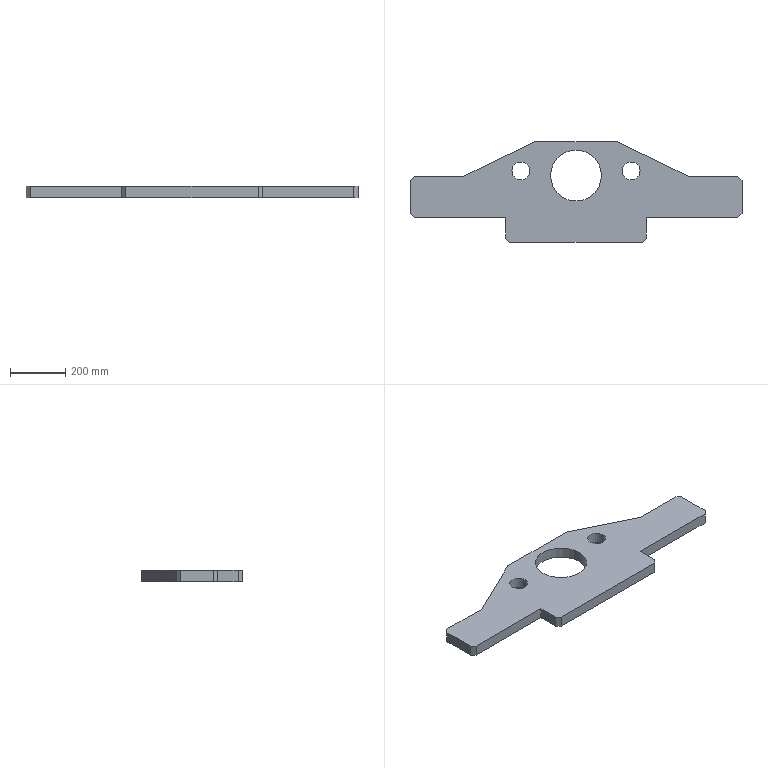Part | SolidWorks | features Extrusion 1 | 1 solid | 26 faces | box 1205 x 365 x 40 mm | volume 10483325 mm3 | plane 20 | cylinder 6 | commonest cylinder face diameters 65 x4 185 x2
STEP:
#1=CARTESIAN_POINT('',(-92.5,242.,40.));
#2=VERTEX_POINT('',#1);
#3=CARTESIAN_POINT('',(92.5,242.,40.));
#4=VERTEX_POINT('',#3);
#5=CARTESIAN_POINT('',(0.,242.,40.));
#6=DIRECTION('',(0.,0.,1.));
#7=DIRECTION('',(1.,0.,0.));
#8=AXIS2_PLACEMENT_3D('',#5,#6,#7);
#9=CIRCLE('',#8,92.5);
#10=EDGE_CURVE('',#2,#4,#9,.T.);
#11=ORIENTED_EDGE('',*,*,#10,.T.);
#12=CARTESIAN_POINT('',(92.5,242.,0.));
#13=VERTEX_POINT('',#12);
#14=CARTESIAN_POINT('',(92.5,242.,40.));
#15=DIRECTION('',(0.,0.,-1.));
#16=VECTOR('',#15,1000.);
#17=LINE('',#14,#16);
#18=EDGE_CURVE('',#4,#13,#17,.T.);
#19=ORIENTED_EDGE('',*,*,#18,.T.);
#20=CARTESIAN_POINT('',(-92.5,242.,0.));
#21=VERTEX_POINT('',#20);
#22=CARTESIAN_POINT('',(0.,242.,0.));
#23=DIRECTION('',(0.,0.,1.));
#24=DIRECTION('',(1.,0.,0.));
#25=AXIS2_PLACEMENT_3D('',#22,#23,#24);
#26=CIRCLE('',#25,92.5);
#27=EDGE_CURVE('',#21,#13,#26,.T.);
#28=ORIENTED_EDGE('',*,*,#27,.F.);
#29=CARTESIAN_POINT('',(-92.5,242.,40.));
#30=DIRECTION('',(0.,0.,-1.));
#31=VECTOR('',#30,1000.);
#32=LINE('',#29,#31);
#33=EDGE_CURVE('',#2,#21,#32,.T.);
#34=ORIENTED_EDGE('',*,*,#33,.F.);
#35=EDGE_LOOP('',(#11,#19,#28,#34));
#36=FACE_OUTER_BOUND('',#35,.T.);
#37=CARTESIAN_POINT('',(0.,242.,40.));
#38=DIRECTION('',(0.,0.,-1.));
#39=DIRECTION('',(-1.,0.,0.));
#40=AXIS2_PLACEMENT_3D('',#37,#38,#39);
#41=CYLINDRICAL_SURFACE('',#40,92.5);
#42=ADVANCED_FACE('',(#36),#41,.F.);
#43=CARTESIAN_POINT('',(167.5,259.,40.));
#44=VERTEX_POINT('',#43);
#45=CARTESIAN_POINT('',(232.5,259.,40.));
#46=VERTEX_POINT('',#45);
#47=CARTESIAN_POINT('',(200.,259.,40.));
#48=DIRECTION('',(0.,0.,1.));
#49=DIRECTION('',(-1.,0.,0.));
#50=AXIS2_PLACEMENT_3D('',#47,#48,#49);
#51=CIRCLE('',#50,32.5);
#52=EDGE_CURVE('',#44,#46,#51,.T.);
#53=ORIENTED_EDGE('',*,*,#52,.T.);
#54=CARTESIAN_POINT('',(232.5,259.,0.));
#55=VERTEX_POINT('',#54);
#56=CARTESIAN_POINT('',(232.5,259.,40.));
#57=DIRECTION('',(0.,0.,-1.));
#58=VECTOR('',#57,1000.);
#59=LINE('',#56,#58);
#60=EDGE_CURVE('',#46,#55,#59,.T.);
#61=ORIENTED_EDGE('',*,*,#60,.T.);
#62=CARTESIAN_POINT('',(167.5,259.,0.));
#63=VERTEX_POINT('',#62);
#64=CARTESIAN_POINT('',(200.,259.,0.));
#65=DIRECTION('',(0.,0.,1.));
#66=DIRECTION('',(-1.,0.,0.));
#67=AXIS2_PLACEMENT_3D('',#64,#65,#66);
#68=CIRCLE('',#67,32.5);
#69=EDGE_CURVE('',#63,#55,#68,.T.);
#70=ORIENTED_EDGE('',*,*,#69,.F.);
#71=CARTESIAN_POINT('',(167.5,259.,40.));
#72=DIRECTION('',(0.,0.,-1.));
#73=VECTOR('',#72,1000.);
#74=LINE('',#71,#73);
#75=EDGE_CURVE('',#44,#63,#74,.T.);
#76=ORIENTED_EDGE('',*,*,#75,.F.);
#77=EDGE_LOOP('',(#53,#61,#70,#76));
#78=FACE_OUTER_BOUND('',#77,.T.);
#79=CARTESIAN_POINT('',(200.,259.,40.));
#80=DIRECTION('',(0.,0.,-1.));
#81=DIRECTION('',(-1.,0.,0.));
#82=AXIS2_PLACEMENT_3D('',#79,#80,#81);
#83=CYLINDRICAL_SURFACE('',#82,32.5);
#84=ADVANCED_FACE('',(#78),#83,.F.);
#85=CARTESIAN_POINT('',(-232.5,259.,40.));
#86=VERTEX_POINT('',#85);
#87=CARTESIAN_POINT('',(-167.5,259.,40.));
#88=VERTEX_POINT('',#87);
#89=CARTESIAN_POINT('',(-200.,259.,40.));
#90=DIRECTION('',(0.,0.,1.));
#91=DIRECTION('',(1.,0.,0.));
#92=AXIS2_PLACEMENT_3D('',#89,#90,#91);
#93=CIRCLE('',#92,32.5);
#94=EDGE_CURVE('',#86,#88,#93,.T.);
#95=ORIENTED_EDGE('',*,*,#94,.T.);
#96=CARTESIAN_POINT('',(-167.5,259.,0.));
#97=VERTEX_POINT('',#96);
#98=CARTESIAN_POINT('',(-167.5,259.,40.));
#99=DIRECTION('',(0.,0.,-1.));
#100=VECTOR('',#99,1000.);
#101=LINE('',#98,#100);
#102=EDGE_CURVE('',#88,#97,#101,.T.);
#103=ORIENTED_EDGE('',*,*,#102,.T.);
#104=CARTESIAN_POINT('',(-232.5,259.,0.));
#105=VERTEX_POINT('',#104);
#106=CARTESIAN_POINT('',(-200.,259.,0.));
#107=DIRECTION('',(0.,0.,1.));
#108=DIRECTION('',(1.,0.,0.));
#109=AXIS2_PLACEMENT_3D('',#106,#107,#108);
#110=CIRCLE('',#109,32.5);
#111=EDGE_CURVE('',#105,#97,#110,.T.);
#112=ORIENTED_EDGE('',*,*,#111,.F.);
#113=CARTESIAN_POINT('',(-232.5,259.,40.));
#114=DIRECTION('',(0.,0.,-1.));
#115=VECTOR('',#114,1000.);
#116=LINE('',#113,#115);
#117=EDGE_CURVE('',#86,#105,#116,.T.);
#118=ORIENTED_EDGE('',*,*,#117,.F.);
#119=EDGE_LOOP('',(#95,#103,#112,#118));
#120=FACE_OUTER_BOUND('',#119,.T.);
#121=CARTESIAN_POINT('',(-200.,259.,40.));
#122=DIRECTION('',(0.,0.,-1.));
#123=DIRECTION('',(-1.,0.,0.));
#124=AXIS2_PLACEMENT_3D('',#121,#122,#123);
#125=CYLINDRICAL_SURFACE('',#124,32.5);
#126=ADVANCED_FACE('',(#120),#125,.F.);
#127=CARTESIAN_POINT('',(-587.5,90.,40.));
#128=VERTEX_POINT('',#127);
#129=CARTESIAN_POINT('',(-255.,90.,40.));
#130=VERTEX_POINT('',#129);
#131=CARTESIAN_POINT('',(-255.,90.,40.));
#132=DIRECTION('',(1.,0.,0.));
#133=VECTOR('',#132,1000.);
#134=LINE('',#131,#133);
#135=EDGE_CURVE('',#128,#130,#134,.T.);
#136=ORIENTED_EDGE('',*,*,#135,.T.);
#137=CARTESIAN_POINT('',(-255.,15.,40.));
#138=VERTEX_POINT('',#137);
#139=CARTESIAN_POINT('',(-255.,15.,40.));
#140=DIRECTION('',(0.,-1.,0.));
#141=VECTOR('',#140,1000.);
#142=LINE('',#139,#141);
#143=EDGE_CURVE('',#130,#138,#142,.T.);
#144=ORIENTED_EDGE('',*,*,#143,.T.);
#145=CARTESIAN_POINT('',(-240.,0.,40.));
#146=VERTEX_POINT('',#145);
#147=CARTESIAN_POINT('',(-240.,0.,40.));
#148=DIRECTION('',(0.7071,-0.7071,0.));
#149=VECTOR('',#148,1000.);
#150=LINE('',#147,#149);
#151=EDGE_CURVE('',#138,#146,#150,.T.);
#152=ORIENTED_EDGE('',*,*,#151,.T.);
#153=CARTESIAN_POINT('',(240.,0.,40.));
#154=VERTEX_POINT('',#153);
#155=CARTESIAN_POINT('',(240.,0.,40.));
#156=DIRECTION('',(1.,0.,0.));
#157=VECTOR('',#156,1000.);
#158=LINE('',#155,#157);
#159=EDGE_CURVE('',#146,#154,#158,.T.);
#160=ORIENTED_EDGE('',*,*,#159,.T.);
#161=CARTESIAN_POINT('',(255.,15.,40.));
#162=VERTEX_POINT('',#161);
#163=CARTESIAN_POINT('',(240.,0.,40.));
#164=DIRECTION('',(0.7071,0.7071,0.));
#165=VECTOR('',#164,1000.);
#166=LINE('',#163,#165);
#167=EDGE_CURVE('',#154,#162,#166,.T.);
#168=ORIENTED_EDGE('',*,*,#167,.T.);
#169=CARTESIAN_POINT('',(255.,90.,40.));
#170=VERTEX_POINT('',#169);
#171=CARTESIAN_POINT('',(255.,15.,40.));
#172=DIRECTION('',(0.,1.,0.));
#173=VECTOR('',#172,1000.);
#174=LINE('',#171,#173);
#175=EDGE_CURVE('',#162,#170,#174,.T.);
#176=ORIENTED_EDGE('',*,*,#175,.T.);
#177=CARTESIAN_POINT('',(587.5,90.,40.));
#178=VERTEX_POINT('',#177);
#179=CARTESIAN_POINT('',(255.,90.,40.));
#180=DIRECTION('',(1.,0.,0.));
#181=VECTOR('',#180,1000.);
#182=LINE('',#179,#181);
#183=EDGE_CURVE('',#170,#178,#182,.T.);
#184=ORIENTED_EDGE('',*,*,#183,.T.);
#185=CARTESIAN_POINT('',(602.5,105.,40.));
#186=VERTEX_POINT('',#185);
#187=CARTESIAN_POINT('',(587.5,90.,40.));
#188=DIRECTION('',(0.7071,0.7071,0.));
#189=VECTOR('',#188,1000.);
#190=LINE('',#187,#189);
#191=EDGE_CURVE('',#178,#186,#190,.T.);
#192=ORIENTED_EDGE('',*,*,#191,.T.);
#193=CARTESIAN_POINT('',(602.5,225.,40.));
#194=VERTEX_POINT('',#193);
#195=CARTESIAN_POINT('',(602.5,105.,40.));
#196=DIRECTION('',(0.,1.,0.));
#197=VECTOR('',#196,1000.);
#198=LINE('',#195,#197);
#199=EDGE_CURVE('',#186,#194,#198,.T.);
#200=ORIENTED_EDGE('',*,*,#199,.T.);
#201=CARTESIAN_POINT('',(587.5,240.,40.));
#202=VERTEX_POINT('',#201);
#203=CARTESIAN_POINT('',(602.5,225.,40.));
#204=DIRECTION('',(-0.7071,0.7071,0.));
#205=VECTOR('',#204,1000.);
#206=LINE('',#203,#205);
#207=EDGE_CURVE('',#194,#202,#206,.T.);
#208=ORIENTED_EDGE('',*,*,#207,.T.);
#209=CARTESIAN_POINT('',(407.,240.,40.));
#210=VERTEX_POINT('',#209);
#211=CARTESIAN_POINT('',(587.5,240.,40.));
#212=DIRECTION('',(-1.,0.,0.));
#213=VECTOR('',#212,1000.);
#214=LINE('',#211,#213);
#215=EDGE_CURVE('',#202,#210,#214,.T.);
#216=ORIENTED_EDGE('',*,*,#215,.T.);
#217=CARTESIAN_POINT('',(150.,365.,40.));
#218=VERTEX_POINT('',#217);
#219=CARTESIAN_POINT('',(407.,240.,40.));
#220=DIRECTION('',(-0.8993,0.4374,0.));
#221=VECTOR('',#220,1000.);
#222=LINE('',#219,#221);
#223=EDGE_CURVE('',#210,#218,#222,.T.);
#224=ORIENTED_EDGE('',*,*,#223,.T.);
#225=CARTESIAN_POINT('',(-150.,365.,40.));
#226=VERTEX_POINT('',#225);
#227=CARTESIAN_POINT('',(-150.,365.,40.));
#228=DIRECTION('',(-1.,0.,0.));
#229=VECTOR('',#228,1000.);
#230=LINE('',#227,#229);
#231=EDGE_CURVE('',#218,#226,#230,.T.);
#232=ORIENTED_EDGE('',*,*,#231,.T.);
#233=CARTESIAN_POINT('',(-407.,240.,40.));
#234=VERTEX_POINT('',#233);
#235=CARTESIAN_POINT('',(-407.,240.,40.));
#236=DIRECTION('',(-0.8993,-0.4374,0.));
#237=VECTOR('',#236,1000.);
#238=LINE('',#235,#237);
#239=EDGE_CURVE('',#226,#234,#238,.T.);
#240=ORIENTED_EDGE('',*,*,#239,.T.);
#241=CARTESIAN_POINT('',(-587.5,240.,40.));
#242=VERTEX_POINT('',#241);
#243=CARTESIAN_POINT('',(-587.5,240.,40.));
#244=DIRECTION('',(-1.,0.,0.));
#245=VECTOR('',#244,1000.);
#246=LINE('',#243,#245);
#247=EDGE_CURVE('',#234,#242,#246,.T.);
#248=ORIENTED_EDGE('',*,*,#247,.T.);
#249=CARTESIAN_POINT('',(-602.5,225.,40.));
#250=VERTEX_POINT('',#249);
#251=CARTESIAN_POINT('',(-602.5,225.,40.));
#252=DIRECTION('',(-0.7071,-0.7071,0.));
#253=VECTOR('',#252,1000.);
#254=LINE('',#251,#253);
#255=EDGE_CURVE('',#242,#250,#254,.T.);
#256=ORIENTED_EDGE('',*,*,#255,.T.);
#257=CARTESIAN_POINT('',(-602.5,105.,40.));
#258=VERTEX_POINT('',#257);
#259=CARTESIAN_POINT('',(-602.5,105.,40.));
#260=DIRECTION('',(0.,-1.,0.));
#261=VECTOR('',#260,1000.);
#262=LINE('',#259,#261);
#263=EDGE_CURVE('',#250,#258,#262,.T.);
#264=ORIENTED_EDGE('',*,*,#263,.T.);
#265=CARTESIAN_POINT('',(-587.5,90.,40.));
#266=DIRECTION('',(0.7071,-0.7071,0.));
#267=VECTOR('',#266,1000.);
#268=LINE('',#265,#267);
#269=EDGE_CURVE('',#258,#128,#268,.T.);
#270=ORIENTED_EDGE('',*,*,#269,.T.);
#271=EDGE_LOOP('',(#136,#144,#152,#160,#168,#176,#184,#192,#200,#208,#216,#224,#232,#240,#248,#256,#264,#270));
#272=FACE_OUTER_BOUND('',#271,.T.);
#273=ORIENTED_EDGE('',*,*,#94,.F.);
#274=CARTESIAN_POINT('',(-200.,259.,40.));
#275=DIRECTION('',(0.,0.,1.));
#276=DIRECTION('',(1.,0.,0.));
#277=AXIS2_PLACEMENT_3D('',#274,#275,#276);
#278=CIRCLE('',#277,32.5);
#279=EDGE_CURVE('',#88,#86,#278,.T.);
#280=ORIENTED_EDGE('',*,*,#279,.F.);
#281=EDGE_LOOP('',(#273,#280));
#282=FACE_BOUND('',#281,.T.);
#283=ORIENTED_EDGE('',*,*,#52,.F.);
#284=CARTESIAN_POINT('',(200.,259.,40.));
#285=DIRECTION('',(0.,0.,1.));
#286=DIRECTION('',(-1.,0.,0.));
#287=AXIS2_PLACEMENT_3D('',#284,#285,#286);
#288=CIRCLE('',#287,32.5);
#289=EDGE_CURVE('',#46,#44,#288,.T.);
#290=ORIENTED_EDGE('',*,*,#289,.F.);
#291=EDGE_LOOP('',(#283,#290));
#292=FACE_BOUND('',#291,.T.);
#293=ORIENTED_EDGE('',*,*,#10,.F.);
#294=CARTESIAN_POINT('',(0.,242.,40.));
#295=DIRECTION('',(0.,0.,1.));
#296=DIRECTION('',(1.,0.,0.));
#297=AXIS2_PLACEMENT_3D('',#294,#295,#296);
#298=CIRCLE('',#297,92.5);
#299=EDGE_CURVE('',#4,#2,#298,.T.);
#300=ORIENTED_EDGE('',*,*,#299,.F.);
#301=EDGE_LOOP('',(#293,#300));
#302=FACE_BOUND('',#301,.T.);
#303=CARTESIAN_POINT('',(0.,0.,40.));
#304=DIRECTION('',(0.,0.,-1.));
#305=DIRECTION('',(-1.,0.,0.));
#306=AXIS2_PLACEMENT_3D('',#303,#304,#305);
#307=PLANE('',#306);
#308=ADVANCED_FACE('',(#272,#282,#292,#302),#307,.F.);
#309=ORIENTED_EDGE('',*,*,#69,.T.);
#310=CARTESIAN_POINT('',(200.,259.,0.));
#311=DIRECTION('',(0.,0.,1.));
#312=DIRECTION('',(-1.,0.,0.));
#313=AXIS2_PLACEMENT_3D('',#310,#311,#312);
#314=CIRCLE('',#313,32.5);
#315=EDGE_CURVE('',#55,#63,#314,.T.);
#316=ORIENTED_EDGE('',*,*,#315,.T.);
#317=EDGE_LOOP('',(#309,#316));
#318=FACE_BOUND('',#317,.T.);
#319=CARTESIAN_POINT('',(-587.5,90.,0.));
#320=VERTEX_POINT('',#319);
#321=CARTESIAN_POINT('',(-255.,90.,0.));
#322=VERTEX_POINT('',#321);
#323=CARTESIAN_POINT('',(-255.,90.,0.));
#324=DIRECTION('',(1.,0.,0.));
#325=VECTOR('',#324,1000.);
#326=LINE('',#323,#325);
#327=EDGE_CURVE('',#320,#322,#326,.T.);
#328=ORIENTED_EDGE('',*,*,#327,.F.);
#329=CARTESIAN_POINT('',(-602.5,105.,0.));
#330=VERTEX_POINT('',#329);
#331=CARTESIAN_POINT('',(-587.5,90.,0.));
#332=DIRECTION('',(0.7071,-0.7071,0.));
#333=VECTOR('',#332,1000.);
#334=LINE('',#331,#333);
#335=EDGE_CURVE('',#330,#320,#334,.T.);
#336=ORIENTED_EDGE('',*,*,#335,.F.);
#337=CARTESIAN_POINT('',(-602.5,225.,0.));
#338=VERTEX_POINT('',#337);
#339=CARTESIAN_POINT('',(-602.5,105.,0.));
#340=DIRECTION('',(0.,-1.,0.));
#341=VECTOR('',#340,1000.);
#342=LINE('',#339,#341);
#343=EDGE_CURVE('',#338,#330,#342,.T.);
#344=ORIENTED_EDGE('',*,*,#343,.F.);
#345=CARTESIAN_POINT('',(-587.5,240.,0.));
#346=VERTEX_POINT('',#345);
#347=CARTESIAN_POINT('',(-602.5,225.,0.));
#348=DIRECTION('',(-0.7071,-0.7071,0.));
#349=VECTOR('',#348,1000.);
#350=LINE('',#347,#349);
#351=EDGE_CURVE('',#346,#338,#350,.T.);
#352=ORIENTED_EDGE('',*,*,#351,.F.);
#353=CARTESIAN_POINT('',(-407.,240.,0.));
#354=VERTEX_POINT('',#353);
#355=CARTESIAN_POINT('',(-587.5,240.,0.));
#356=DIRECTION('',(-1.,0.,0.));
#357=VECTOR('',#356,1000.);
#358=LINE('',#355,#357);
#359=EDGE_CURVE('',#354,#346,#358,.T.);
#360=ORIENTED_EDGE('',*,*,#359,.F.);
#361=CARTESIAN_POINT('',(-150.,365.,0.));
#362=VERTEX_POINT('',#361);
#363=CARTESIAN_POINT('',(-407.,240.,0.));
#364=DIRECTION('',(-0.8993,-0.4374,0.));
#365=VECTOR('',#364,1000.);
#366=LINE('',#363,#365);
#367=EDGE_CURVE('',#362,#354,#366,.T.);
#368=ORIENTED_EDGE('',*,*,#367,.F.);
#369=CARTESIAN_POINT('',(150.,365.,0.));
#370=VERTEX_POINT('',#369);
#371=CARTESIAN_POINT('',(-150.,365.,0.));
#372=DIRECTION('',(-1.,0.,0.));
#373=VECTOR('',#372,1000.);
#374=LINE('',#371,#373);
#375=EDGE_CURVE('',#370,#362,#374,.T.);
#376=ORIENTED_EDGE('',*,*,#375,.F.);
#377=CARTESIAN_POINT('',(407.,240.,0.));
#378=VERTEX_POINT('',#377);
#379=CARTESIAN_POINT('',(407.,240.,0.));
#380=DIRECTION('',(-0.8993,0.4374,0.));
#381=VECTOR('',#380,1000.);
#382=LINE('',#379,#381);
#383=EDGE_CURVE('',#378,#370,#382,.T.);
#384=ORIENTED_EDGE('',*,*,#383,.F.);
#385=CARTESIAN_POINT('',(587.5,240.,0.));
#386=VERTEX_POINT('',#385);
#387=CARTESIAN_POINT('',(587.5,240.,0.));
#388=DIRECTION('',(-1.,0.,0.));
#389=VECTOR('',#388,1000.);
#390=LINE('',#387,#389);
#391=EDGE_CURVE('',#386,#378,#390,.T.);
#392=ORIENTED_EDGE('',*,*,#391,.F.);
#393=CARTESIAN_POINT('',(602.5,225.,0.));
#394=VERTEX_POINT('',#393);
#395=CARTESIAN_POINT('',(602.5,225.,0.));
#396=DIRECTION('',(-0.7071,0.7071,0.));
#397=VECTOR('',#396,1000.);
#398=LINE('',#395,#397);
#399=EDGE_CURVE('',#394,#386,#398,.T.);
#400=ORIENTED_EDGE('',*,*,#399,.F.);
#401=CARTESIAN_POINT('',(602.5,105.,0.));
#402=VERTEX_POINT('',#401);
#403=CARTESIAN_POINT('',(602.5,105.,0.));
#404=DIRECTION('',(0.,1.,0.));
#405=VECTOR('',#404,1000.);
#406=LINE('',#403,#405);
#407=EDGE_CURVE('',#402,#394,#406,.T.);
#408=ORIENTED_EDGE('',*,*,#407,.F.);
#409=CARTESIAN_POINT('',(587.5,90.,0.));
#410=VERTEX_POINT('',#409);
#411=CARTESIAN_POINT('',(587.5,90.,0.));
#412=DIRECTION('',(0.7071,0.7071,0.));
#413=VECTOR('',#412,1000.);
#414=LINE('',#411,#413);
#415=EDGE_CURVE('',#410,#402,#414,.T.);
#416=ORIENTED_EDGE('',*,*,#415,.F.);
#417=CARTESIAN_POINT('',(255.,90.,0.));
#418=VERTEX_POINT('',#417);
#419=CARTESIAN_POINT('',(255.,90.,0.));
#420=DIRECTION('',(1.,0.,0.));
#421=VECTOR('',#420,1000.);
#422=LINE('',#419,#421);
#423=EDGE_CURVE('',#418,#410,#422,.T.);
#424=ORIENTED_EDGE('',*,*,#423,.F.);
#425=CARTESIAN_POINT('',(255.,15.,0.));
#426=VERTEX_POINT('',#425);
#427=CARTESIAN_POINT('',(255.,15.,0.));
#428=DIRECTION('',(0.,1.,0.));
#429=VECTOR('',#428,1000.);
#430=LINE('',#427,#429);
#431=EDGE_CURVE('',#426,#418,#430,.T.);
#432=ORIENTED_EDGE('',*,*,#431,.F.);
#433=CARTESIAN_POINT('',(240.,0.,0.));
#434=VERTEX_POINT('',#433);
#435=CARTESIAN_POINT('',(240.,0.,0.));
#436=DIRECTION('',(0.7071,0.7071,0.));
#437=VECTOR('',#436,1000.);
#438=LINE('',#435,#437);
#439=EDGE_CURVE('',#434,#426,#438,.T.);
#440=ORIENTED_EDGE('',*,*,#439,.F.);
#441=CARTESIAN_POINT('',(-240.,0.,0.));
#442=VERTEX_POINT('',#441);
#443=CARTESIAN_POINT('',(240.,0.,0.));
#444=DIRECTION('',(1.,0.,0.));
#445=VECTOR('',#444,1000.);
#446=LINE('',#443,#445);
#447=EDGE_CURVE('',#442,#434,#446,.T.);
#448=ORIENTED_EDGE('',*,*,#447,.F.);
#449=CARTESIAN_POINT('',(-255.,15.,0.));
#450=VERTEX_POINT('',#449);
#451=CARTESIAN_POINT('',(-240.,0.,0.));
#452=DIRECTION('',(0.7071,-0.7071,0.));
#453=VECTOR('',#452,1000.);
#454=LINE('',#451,#453);
#455=EDGE_CURVE('',#450,#442,#454,.T.);
#456=ORIENTED_EDGE('',*,*,#455,.F.);
#457=CARTESIAN_POINT('',(-255.,15.,0.));
#458=DIRECTION('',(0.,-1.,0.));
#459=VECTOR('',#458,1000.);
#460=LINE('',#457,#459);
#461=EDGE_CURVE('',#322,#450,#460,.T.);
#462=ORIENTED_EDGE('',*,*,#461,.F.);
#463=EDGE_LOOP('',(#328,#336,#344,#352,#360,#368,#376,#384,#392,#400,#408,#416,#424,#432,#440,#448,#456,#462));
#464=FACE_OUTER_BOUND('',#463,.T.);
#465=ORIENTED_EDGE('',*,*,#111,.T.);
#466=CARTESIAN_POINT('',(-200.,259.,0.));
#467=DIRECTION('',(0.,0.,1.));
#468=DIRECTION('',(1.,0.,0.));
#469=AXIS2_PLACEMENT_3D('',#466,#467,#468);
#470=CIRCLE('',#469,32.5);
#471=EDGE_CURVE('',#97,#105,#470,.T.);
#472=ORIENTED_EDGE('',*,*,#471,.T.);
#473=EDGE_LOOP('',(#465,#472));
#474=FACE_BOUND('',#473,.T.);
#475=ORIENTED_EDGE('',*,*,#27,.T.);
#476=CARTESIAN_POINT('',(0.,242.,0.));
#477=DIRECTION('',(0.,0.,1.));
#478=DIRECTION('',(1.,0.,0.));
#479=AXIS2_PLACEMENT_3D('',#476,#477,#478);
#480=CIRCLE('',#479,92.5);
#481=EDGE_CURVE('',#13,#21,#480,.T.);
#482=ORIENTED_EDGE('',*,*,#481,.T.);
#483=EDGE_LOOP('',(#475,#482));
#484=FACE_BOUND('',#483,.T.);
#485=CARTESIAN_POINT('',(0.,0.,0.));
#486=DIRECTION('',(0.,0.,-1.));
#487=DIRECTION('',(-1.,0.,0.));
#488=AXIS2_PLACEMENT_3D('',#485,#486,#487);
#489=PLANE('',#488);
#490=ADVANCED_FACE('',(#318,#464,#474,#484),#489,.T.);
#491=ORIENTED_EDGE('',*,*,#327,.T.);
#492=CARTESIAN_POINT('',(-255.,90.,40.));
#493=DIRECTION('',(0.,0.,-1.));
#494=VECTOR('',#493,1000.);
#495=LINE('',#492,#494);
#496=EDGE_CURVE('',#130,#322,#495,.T.);
#497=ORIENTED_EDGE('',*,*,#496,.F.);
#498=ORIENTED_EDGE('',*,*,#135,.F.);
#499=CARTESIAN_POINT('',(-587.5,90.,40.));
#500=DIRECTION('',(0.,0.,-1.));
#501=VECTOR('',#500,1000.);
#502=LINE('',#499,#501);
#503=EDGE_CURVE('',#128,#320,#502,.T.);
#504=ORIENTED_EDGE('',*,*,#503,.T.);
#505=EDGE_LOOP('',(#491,#497,#498,#504));
#506=FACE_OUTER_BOUND('',#505,.T.);
#507=CARTESIAN_POINT('',(-255.,90.,40.));
#508=DIRECTION('',(0.,1.,0.));
#509=DIRECTION('',(-1.,0.,0.));
#510=AXIS2_PLACEMENT_3D('',#507,#508,#509);
#511=PLANE('',#510);
#512=ADVANCED_FACE('',(#506),#511,.F.);
#513=ORIENTED_EDGE('',*,*,#461,.T.);
#514=CARTESIAN_POINT('',(-255.,15.,40.));
#515=DIRECTION('',(0.,0.,-1.));
#516=VECTOR('',#515,1000.);
#517=LINE('',#514,#516);
#518=EDGE_CURVE('',#138,#450,#517,.T.);
#519=ORIENTED_EDGE('',*,*,#518,.F.);
#520=ORIENTED_EDGE('',*,*,#143,.F.);
#521=ORIENTED_EDGE('',*,*,#496,.T.);
#522=EDGE_LOOP('',(#513,#519,#520,#521));
#523=FACE_OUTER_BOUND('',#522,.T.);
#524=CARTESIAN_POINT('',(-255.,15.,40.));
#525=DIRECTION('',(1.,0.,0.));
#526=DIRECTION('',(0.,0.,-1.));
#527=AXIS2_PLACEMENT_3D('',#524,#525,#526);
#528=PLANE('',#527);
#529=ADVANCED_FACE('',(#523),#528,.F.);
#530=ORIENTED_EDGE('',*,*,#455,.T.);
#531=CARTESIAN_POINT('',(-240.,0.,40.));
#532=DIRECTION('',(0.,0.,-1.));
#533=VECTOR('',#532,1000.);
#534=LINE('',#531,#533);
#535=EDGE_CURVE('',#146,#442,#534,.T.);
#536=ORIENTED_EDGE('',*,*,#535,.F.);
#537=ORIENTED_EDGE('',*,*,#151,.F.);
#538=ORIENTED_EDGE('',*,*,#518,.T.);
#539=EDGE_LOOP('',(#530,#536,#537,#538));
#540=FACE_OUTER_BOUND('',#539,.T.);
#541=CARTESIAN_POINT('',(-240.,0.,40.));
#542=DIRECTION('',(0.7071,0.7071,0.));
#543=DIRECTION('',(-0.7071,0.7071,0.));
#544=AXIS2_PLACEMENT_3D('',#541,#542,#543);
#545=PLANE('',#544);
#546=ADVANCED_FACE('',(#540),#545,.F.);
#547=ORIENTED_EDGE('',*,*,#447,.T.);
#548=CARTESIAN_POINT('',(240.,0.,40.));
#549=DIRECTION('',(0.,0.,-1.));
#550=VECTOR('',#549,1000.);
#551=LINE('',#548,#550);
#552=EDGE_CURVE('',#154,#434,#551,.T.);
#553=ORIENTED_EDGE('',*,*,#552,.F.);
#554=ORIENTED_EDGE('',*,*,#159,.F.);
#555=ORIENTED_EDGE('',*,*,#535,.T.);
#556=EDGE_LOOP('',(#547,#553,#554,#555));
#557=FACE_OUTER_BOUND('',#556,.T.);
#558=CARTESIAN_POINT('',(240.,0.,40.));
#559=DIRECTION('',(0.,1.,0.));
#560=DIRECTION('',(-1.,0.,0.));
#561=AXIS2_PLACEMENT_3D('',#558,#559,#560);
#562=PLANE('',#561);
#563=ADVANCED_FACE('',(#557),#562,.F.);
#564=ORIENTED_EDGE('',*,*,#439,.T.);
#565=CARTESIAN_POINT('',(255.,15.,40.));
#566=DIRECTION('',(0.,0.,-1.));
#567=VECTOR('',#566,1000.);
#568=LINE('',#565,#567);
#569=EDGE_CURVE('',#162,#426,#568,.T.);
#570=ORIENTED_EDGE('',*,*,#569,.F.);
#571=ORIENTED_EDGE('',*,*,#167,.F.);
#572=ORIENTED_EDGE('',*,*,#552,.T.);
#573=EDGE_LOOP('',(#564,#570,#571,#572));
#574=FACE_OUTER_BOUND('',#573,.T.);
#575=CARTESIAN_POINT('',(240.,0.,40.));
#576=DIRECTION('',(-0.7071,0.7071,0.));
#577=DIRECTION('',(-0.7071,-0.7071,0.));
#578=AXIS2_PLACEMENT_3D('',#575,#576,#577);
#579=PLANE('',#578);
#580=ADVANCED_FACE('',(#574),#579,.F.);
#581=ORIENTED_EDGE('',*,*,#431,.T.);
#582=CARTESIAN_POINT('',(255.,90.,40.));
#583=DIRECTION('',(0.,0.,-1.));
#584=VECTOR('',#583,1000.);
#585=LINE('',#582,#584);
#586=EDGE_CURVE('',#170,#418,#585,.T.);
#587=ORIENTED_EDGE('',*,*,#586,.F.);
#588=ORIENTED_EDGE('',*,*,#175,.F.);
#589=ORIENTED_EDGE('',*,*,#569,.T.);
#590=EDGE_LOOP('',(#581,#587,#588,#589));
#591=FACE_OUTER_BOUND('',#590,.T.);
#592=CARTESIAN_POINT('',(255.,15.,40.));
#593=DIRECTION('',(-1.,0.,0.));
#594=DIRECTION('',(0.,0.,1.));
#595=AXIS2_PLACEMENT_3D('',#592,#593,#594);
#596=PLANE('',#595);
#597=ADVANCED_FACE('',(#591),#596,.F.);
#598=ORIENTED_EDGE('',*,*,#423,.T.);
#599=CARTESIAN_POINT('',(587.5,90.,40.));
#600=DIRECTION('',(0.,0.,-1.));
#601=VECTOR('',#600,1000.);
#602=LINE('',#599,#601);
#603=EDGE_CURVE('',#178,#410,#602,.T.);
#604=ORIENTED_EDGE('',*,*,#603,.F.);
#605=ORIENTED_EDGE('',*,*,#183,.F.);
#606=ORIENTED_EDGE('',*,*,#586,.T.);
#607=EDGE_LOOP('',(#598,#604,#605,#606));
#608=FACE_OUTER_BOUND('',#607,.T.);
#609=CARTESIAN_POINT('',(255.,90.,40.));
#610=DIRECTION('',(0.,1.,0.));
#611=DIRECTION('',(-1.,0.,0.));
#612=AXIS2_PLACEMENT_3D('',#609,#610,#611);
#613=PLANE('',#612);
#614=ADVANCED_FACE('',(#608),#613,.F.);
#615=ORIENTED_EDGE('',*,*,#415,.T.);
#616=CARTESIAN_POINT('',(602.5,105.,40.));
#617=DIRECTION('',(0.,0.,-1.));
#618=VECTOR('',#617,1000.);
#619=LINE('',#616,#618);
#620=EDGE_CURVE('',#186,#402,#619,.T.);
#621=ORIENTED_EDGE('',*,*,#620,.F.);
#622=ORIENTED_EDGE('',*,*,#191,.F.);
#623=ORIENTED_EDGE('',*,*,#603,.T.);
#624=EDGE_LOOP('',(#615,#621,#622,#623));
#625=FACE_OUTER_BOUND('',#624,.T.);
#626=CARTESIAN_POINT('',(587.5,90.,40.));
#627=DIRECTION('',(-0.7071,0.7071,0.));
#628=DIRECTION('',(-0.7071,-0.7071,0.));
#629=AXIS2_PLACEMENT_3D('',#626,#627,#628);
#630=PLANE('',#629);
#631=ADVANCED_FACE('',(#625),#630,.F.);
#632=ORIENTED_EDGE('',*,*,#407,.T.);
#633=CARTESIAN_POINT('',(602.5,225.,40.));
#634=DIRECTION('',(0.,0.,-1.));
#635=VECTOR('',#634,1000.);
#636=LINE('',#633,#635);
#637=EDGE_CURVE('',#194,#394,#636,.T.);
#638=ORIENTED_EDGE('',*,*,#637,.F.);
#639=ORIENTED_EDGE('',*,*,#199,.F.);
#640=ORIENTED_EDGE('',*,*,#620,.T.);
#641=EDGE_LOOP('',(#632,#638,#639,#640));
#642=FACE_OUTER_BOUND('',#641,.T.);
#643=CARTESIAN_POINT('',(602.5,105.,40.));
#644=DIRECTION('',(-1.,0.,0.));
#645=DIRECTION('',(0.,0.,1.));
#646=AXIS2_PLACEMENT_3D('',#643,#644,#645);
#647=PLANE('',#646);
#648=ADVANCED_FACE('',(#642),#647,.F.);
#649=ORIENTED_EDGE('',*,*,#399,.T.);
#650=CARTESIAN_POINT('',(587.5,240.,40.));
#651=DIRECTION('',(0.,0.,-1.));
#652=VECTOR('',#651,1000.);
#653=LINE('',#650,#652);
#654=EDGE_CURVE('',#202,#386,#653,.T.);
#655=ORIENTED_EDGE('',*,*,#654,.F.);
#656=ORIENTED_EDGE('',*,*,#207,.F.);
#657=ORIENTED_EDGE('',*,*,#637,.T.);
#658=EDGE_LOOP('',(#649,#655,#656,#657));
#659=FACE_OUTER_BOUND('',#658,.T.);
#660=CARTESIAN_POINT('',(602.5,225.,40.));
#661=DIRECTION('',(-0.7071,-0.7071,0.));
#662=DIRECTION('',(0.7071,-0.7071,0.));
#663=AXIS2_PLACEMENT_3D('',#660,#661,#662);
#664=PLANE('',#663);
#665=ADVANCED_FACE('',(#659),#664,.F.);
#666=ORIENTED_EDGE('',*,*,#391,.T.);
#667=CARTESIAN_POINT('',(407.,240.,40.));
#668=DIRECTION('',(0.,0.,-1.));
#669=VECTOR('',#668,1000.);
#670=LINE('',#667,#669);
#671=EDGE_CURVE('',#210,#378,#670,.T.);
#672=ORIENTED_EDGE('',*,*,#671,.F.);
#673=ORIENTED_EDGE('',*,*,#215,.F.);
#674=ORIENTED_EDGE('',*,*,#654,.T.);
#675=EDGE_LOOP('',(#666,#672,#673,#674));
#676=FACE_OUTER_BOUND('',#675,.T.);
#677=CARTESIAN_POINT('',(587.5,240.,40.));
#678=DIRECTION('',(0.,-1.,0.));
#679=DIRECTION('',(1.,0.,0.));
#680=AXIS2_PLACEMENT_3D('',#677,#678,#679);
#681=PLANE('',#680);
#682=ADVANCED_FACE('',(#676),#681,.F.);
#683=ORIENTED_EDGE('',*,*,#383,.T.);
#684=CARTESIAN_POINT('',(150.,365.,40.));
#685=DIRECTION('',(0.,0.,-1.));
#686=VECTOR('',#685,1000.);
#687=LINE('',#684,#686);
#688=EDGE_CURVE('',#218,#370,#687,.T.);
#689=ORIENTED_EDGE('',*,*,#688,.F.);
#690=ORIENTED_EDGE('',*,*,#223,.F.);
#691=ORIENTED_EDGE('',*,*,#671,.T.);
#692=EDGE_LOOP('',(#683,#689,#690,#691));
#693=FACE_OUTER_BOUND('',#692,.T.);
#694=CARTESIAN_POINT('',(407.,240.,40.));
#695=DIRECTION('',(-0.4374,-0.8993,0.));
#696=DIRECTION('',(0.8993,-0.4374,0.));
#697=AXIS2_PLACEMENT_3D('',#694,#695,#696);
#698=PLANE('',#697);
#699=ADVANCED_FACE('',(#693),#698,.F.);
#700=ORIENTED_EDGE('',*,*,#375,.T.);
#701=CARTESIAN_POINT('',(-150.,365.,40.));
#702=DIRECTION('',(0.,0.,-1.));
#703=VECTOR('',#702,1000.);
#704=LINE('',#701,#703);
#705=EDGE_CURVE('',#226,#362,#704,.T.);
#706=ORIENTED_EDGE('',*,*,#705,.F.);
#707=ORIENTED_EDGE('',*,*,#231,.F.);
#708=ORIENTED_EDGE('',*,*,#688,.T.);
#709=EDGE_LOOP('',(#700,#706,#707,#708));
#710=FACE_OUTER_BOUND('',#709,.T.);
#711=CARTESIAN_POINT('',(-150.,365.,40.));
#712=DIRECTION('',(0.,-1.,0.));
#713=DIRECTION('',(1.,0.,0.));
#714=AXIS2_PLACEMENT_3D('',#711,#712,#713);
#715=PLANE('',#714);
#716=ADVANCED_FACE('',(#710),#715,.F.);
#717=ORIENTED_EDGE('',*,*,#367,.T.);
#718=CARTESIAN_POINT('',(-407.,240.,40.));
#719=DIRECTION('',(0.,0.,-1.));
#720=VECTOR('',#719,1000.);
#721=LINE('',#718,#720);
#722=EDGE_CURVE('',#234,#354,#721,.T.);
#723=ORIENTED_EDGE('',*,*,#722,.F.);
#724=ORIENTED_EDGE('',*,*,#239,.F.);
#725=ORIENTED_EDGE('',*,*,#705,.T.);
#726=EDGE_LOOP('',(#717,#723,#724,#725));
#727=FACE_OUTER_BOUND('',#726,.T.);
#728=CARTESIAN_POINT('',(-407.,240.,40.));
#729=DIRECTION('',(0.4374,-0.8993,0.));
#730=DIRECTION('',(0.8993,0.4374,0.));
#731=AXIS2_PLACEMENT_3D('',#728,#729,#730);
#732=PLANE('',#731);
#733=ADVANCED_FACE('',(#727),#732,.F.);
#734=ORIENTED_EDGE('',*,*,#359,.T.);
#735=CARTESIAN_POINT('',(-587.5,240.,40.));
#736=DIRECTION('',(0.,0.,-1.));
#737=VECTOR('',#736,1000.);
#738=LINE('',#735,#737);
#739=EDGE_CURVE('',#242,#346,#738,.T.);
#740=ORIENTED_EDGE('',*,*,#739,.F.);
#741=ORIENTED_EDGE('',*,*,#247,.F.);
#742=ORIENTED_EDGE('',*,*,#722,.T.);
#743=EDGE_LOOP('',(#734,#740,#741,#742));
#744=FACE_OUTER_BOUND('',#743,.T.);
#745=CARTESIAN_POINT('',(-587.5,240.,40.));
#746=DIRECTION('',(0.,-1.,0.));
#747=DIRECTION('',(1.,0.,0.));
#748=AXIS2_PLACEMENT_3D('',#745,#746,#747);
#749=PLANE('',#748);
#750=ADVANCED_FACE('',(#744),#749,.F.);
#751=ORIENTED_EDGE('',*,*,#351,.T.);
#752=CARTESIAN_POINT('',(-602.5,225.,40.));
#753=DIRECTION('',(0.,0.,-1.));
#754=VECTOR('',#753,1000.);
#755=LINE('',#752,#754);
#756=EDGE_CURVE('',#250,#338,#755,.T.);
#757=ORIENTED_EDGE('',*,*,#756,.F.);
#758=ORIENTED_EDGE('',*,*,#255,.F.);
#759=ORIENTED_EDGE('',*,*,#739,.T.);
#760=EDGE_LOOP('',(#751,#757,#758,#759));
#761=FACE_OUTER_BOUND('',#760,.T.);
#762=CARTESIAN_POINT('',(-602.5,225.,40.));
#763=DIRECTION('',(0.7071,-0.7071,0.));
#764=DIRECTION('',(0.7071,0.7071,0.));
#765=AXIS2_PLACEMENT_3D('',#762,#763,#764);
#766=PLANE('',#765);
#767=ADVANCED_FACE('',(#761),#766,.F.);
#768=ORIENTED_EDGE('',*,*,#343,.T.);
#769=CARTESIAN_POINT('',(-602.5,105.,40.));
#770=DIRECTION('',(0.,0.,-1.));
#771=VECTOR('',#770,1000.);
#772=LINE('',#769,#771);
#773=EDGE_CURVE('',#258,#330,#772,.T.);
#774=ORIENTED_EDGE('',*,*,#773,.F.);
#775=ORIENTED_EDGE('',*,*,#263,.F.);
#776=ORIENTED_EDGE('',*,*,#756,.T.);
#777=EDGE_LOOP('',(#768,#774,#775,#776));
#778=FACE_OUTER_BOUND('',#777,.T.);
#779=CARTESIAN_POINT('',(-602.5,105.,40.));
#780=DIRECTION('',(1.,0.,0.));
#781=DIRECTION('',(0.,0.,-1.));
#782=AXIS2_PLACEMENT_3D('',#779,#780,#781);
#783=PLANE('',#782);
#784=ADVANCED_FACE('',(#778),#783,.F.);
#785=ORIENTED_EDGE('',*,*,#335,.T.);
#786=ORIENTED_EDGE('',*,*,#503,.F.);
#787=ORIENTED_EDGE('',*,*,#269,.F.);
#788=ORIENTED_EDGE('',*,*,#773,.T.);
#789=EDGE_LOOP('',(#785,#786,#787,#788));
#790=FACE_OUTER_BOUND('',#789,.T.);
#791=CARTESIAN_POINT('',(-587.5,90.,40.));
#792=DIRECTION('',(0.7071,0.7071,0.));
#793=DIRECTION('',(-0.7071,0.7071,0.));
#794=AXIS2_PLACEMENT_3D('',#791,#792,#793);
#795=PLANE('',#794);
#796=ADVANCED_FACE('',(#790),#795,.F.);
#797=ORIENTED_EDGE('',*,*,#102,.F.);
#798=ORIENTED_EDGE('',*,*,#279,.T.);
#799=ORIENTED_EDGE('',*,*,#117,.T.);
#800=ORIENTED_EDGE('',*,*,#471,.F.);
#801=EDGE_LOOP('',(#797,#798,#799,#800));
#802=FACE_OUTER_BOUND('',#801,.T.);
#803=CARTESIAN_POINT('',(-200.,259.,40.));
#804=DIRECTION('',(0.,0.,-1.));
#805=DIRECTION('',(-1.,0.,0.));
#806=AXIS2_PLACEMENT_3D('',#803,#804,#805);
#807=CYLINDRICAL_SURFACE('',#806,32.5);
#808=ADVANCED_FACE('',(#802),#807,.F.);
#809=ORIENTED_EDGE('',*,*,#60,.F.);
#810=ORIENTED_EDGE('',*,*,#289,.T.);
#811=ORIENTED_EDGE('',*,*,#75,.T.);
#812=ORIENTED_EDGE('',*,*,#315,.F.);
#813=EDGE_LOOP('',(#809,#810,#811,#812));
#814=FACE_OUTER_BOUND('',#813,.T.);
#815=CARTESIAN_POINT('',(200.,259.,40.));
#816=DIRECTION('',(0.,0.,-1.));
#817=DIRECTION('',(-1.,0.,0.));
#818=AXIS2_PLACEMENT_3D('',#815,#816,#817);
#819=CYLINDRICAL_SURFACE('',#818,32.5);
#820=ADVANCED_FACE('',(#814),#819,.F.);
#821=ORIENTED_EDGE('',*,*,#18,.F.);
#822=ORIENTED_EDGE('',*,*,#299,.T.);
#823=ORIENTED_EDGE('',*,*,#33,.T.);
#824=ORIENTED_EDGE('',*,*,#481,.F.);
#825=EDGE_LOOP('',(#821,#822,#823,#824));
#826=FACE_OUTER_BOUND('',#825,.T.);
#827=CARTESIAN_POINT('',(0.,242.,40.));
#828=DIRECTION('',(0.,0.,-1.));
#829=DIRECTION('',(-1.,0.,0.));
#830=AXIS2_PLACEMENT_3D('',#827,#828,#829);
#831=CYLINDRICAL_SURFACE('',#830,92.5);
#832=ADVANCED_FACE('',(#826),#831,.F.);
#833=CLOSED_SHELL('',(#42,#84,#126,#308,#490,#512,#529,#546,#563,#580,#597,#614,#631,#648,#665,#682,#699,#716,#733,#750,#767,#784,#796,#808,#820,#832));
#834=MANIFOLD_SOLID_BREP('',#833);
#835=CARTESIAN_POINT('',(0.,0.,0.));
#836=DIRECTION('',(0.,0.,1.));
#837=DIRECTION('',(1.,0.,0.));
#838=AXIS2_PLACEMENT_3D('',#835,#836,#837);
#839=(LENGTH_UNIT()NAMED_UNIT(*)SI_UNIT(.MILLI.,.METRE.));
#840=UNCERTAINTY_MEASURE_WITH_UNIT(LENGTH_MEASURE(0.00001),#839,'','');
#841=(NAMED_UNIT(*)PLANE_ANGLE_UNIT()SI_UNIT($,.RADIAN.));
#842=(NAMED_UNIT(*)SI_UNIT($,.STERADIAN.)SOLID_ANGLE_UNIT());
#843=(GEOMETRIC_REPRESENTATION_CONTEXT(3)GLOBAL_UNCERTAINTY_ASSIGNED_CONTEXT((#840))GLOBAL_UNIT_ASSIGNED_CONTEXT((#839,#841,#842))REPRESENTATION_CONTEXT('',''));
#844=ADVANCED_BREP_SHAPE_REPRESENTATION('',(#834,#838),#843);